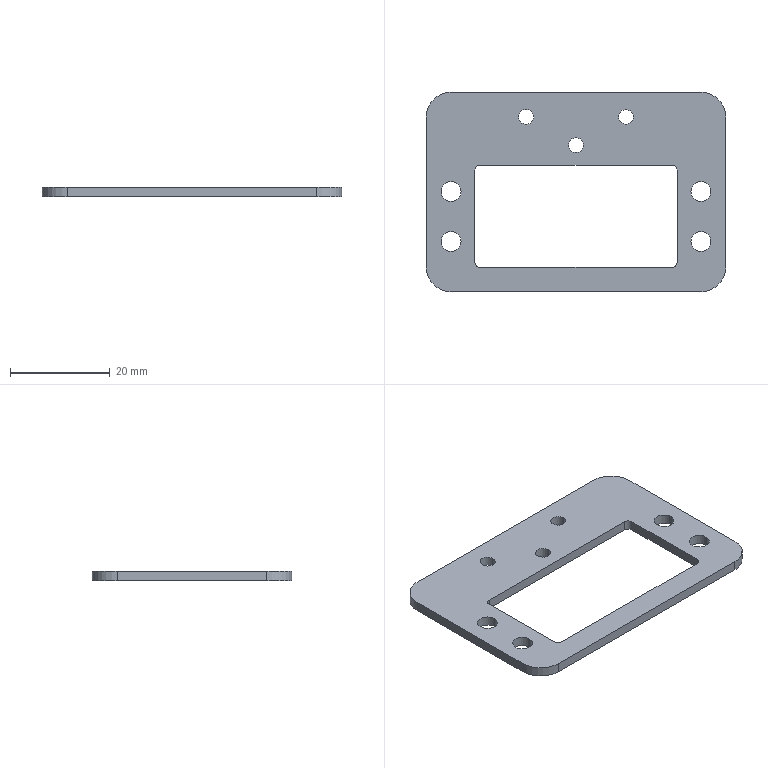Part | SolidWorks | features ICE 3, Extrusion 1 | 1 solid | 32 faces | box 60 x 40 x 2 mm | volume 2957 mm3 | cylinder 22 | plane 10 | commonest cylinder face diameters 4 x8 2 x4 10 x4 2.944 x2 3 x2 3.025 x2
STEP:
#1=CARTESIAN_POINT('',(25.172,6.576,0.));
#2=VERTEX_POINT('',#1);
#3=CARTESIAN_POINT('',(29.172,6.576,0.));
#4=VERTEX_POINT('',#3);
#5=CARTESIAN_POINT('',(27.172,6.576,0.));
#6=DIRECTION('',(0.,0.,1.));
#7=DIRECTION('',(1.,0.,0.));
#8=AXIS2_PLACEMENT_3D('',#5,#6,#7);
#9=CIRCLE('',#8,2.);
#10=EDGE_CURVE('',#2,#4,#9,.T.);
#11=ORIENTED_EDGE('',*,*,#10,.F.);
#12=CARTESIAN_POINT('',(25.172,6.576,2.));
#13=VERTEX_POINT('',#12);
#14=CARTESIAN_POINT('',(25.172,6.576,0.));
#15=DIRECTION('',(0.,0.,1.));
#16=VECTOR('',#15,1000.);
#17=LINE('',#14,#16);
#18=EDGE_CURVE('',#2,#13,#17,.T.);
#19=ORIENTED_EDGE('',*,*,#18,.T.);
#20=CARTESIAN_POINT('',(29.172,6.576,2.));
#21=VERTEX_POINT('',#20);
#22=CARTESIAN_POINT('',(27.172,6.576,2.));
#23=DIRECTION('',(0.,0.,1.));
#24=DIRECTION('',(1.,0.,0.));
#25=AXIS2_PLACEMENT_3D('',#22,#23,#24);
#26=CIRCLE('',#25,2.);
#27=EDGE_CURVE('',#13,#21,#26,.T.);
#28=ORIENTED_EDGE('',*,*,#27,.T.);
#29=CARTESIAN_POINT('',(29.172,6.576,0.));
#30=DIRECTION('',(0.,0.,1.));
#31=VECTOR('',#30,1000.);
#32=LINE('',#29,#31);
#33=EDGE_CURVE('',#4,#21,#32,.T.);
#34=ORIENTED_EDGE('',*,*,#33,.F.);
#35=EDGE_LOOP('',(#11,#19,#28,#34));
#36=FACE_OUTER_BOUND('',#35,.T.);
#37=CARTESIAN_POINT('',(27.172,6.576,0.));
#38=DIRECTION('',(0.,0.,1.));
#39=DIRECTION('',(1.,0.,0.));
#40=AXIS2_PLACEMENT_3D('',#37,#38,#39);
#41=CYLINDRICAL_SURFACE('',#40,2.);
#42=ADVANCED_FACE('',(#36),#41,.F.);
#43=CARTESIAN_POINT('',(-24.859,-3.424,0.));
#44=VERTEX_POINT('',#43);
#45=CARTESIAN_POINT('',(-20.859,-3.424,0.));
#46=VERTEX_POINT('',#45);
#47=CARTESIAN_POINT('',(-22.859,-3.424,0.));
#48=DIRECTION('',(0.,0.,1.));
#49=DIRECTION('',(-1.,0.,0.));
#50=AXIS2_PLACEMENT_3D('',#47,#48,#49);
#51=CIRCLE('',#50,2.);
#52=EDGE_CURVE('',#44,#46,#51,.T.);
#53=ORIENTED_EDGE('',*,*,#52,.F.);
#54=CARTESIAN_POINT('',(-24.859,-3.424,2.));
#55=VERTEX_POINT('',#54);
#56=CARTESIAN_POINT('',(-24.859,-3.424,0.));
#57=DIRECTION('',(0.,0.,1.));
#58=VECTOR('',#57,1000.);
#59=LINE('',#56,#58);
#60=EDGE_CURVE('',#44,#55,#59,.T.);
#61=ORIENTED_EDGE('',*,*,#60,.T.);
#62=CARTESIAN_POINT('',(-20.859,-3.424,2.));
#63=VERTEX_POINT('',#62);
#64=CARTESIAN_POINT('',(-22.859,-3.424,2.));
#65=DIRECTION('',(0.,0.,1.));
#66=DIRECTION('',(-1.,0.,0.));
#67=AXIS2_PLACEMENT_3D('',#64,#65,#66);
#68=CIRCLE('',#67,2.);
#69=EDGE_CURVE('',#55,#63,#68,.T.);
#70=ORIENTED_EDGE('',*,*,#69,.T.);
#71=CARTESIAN_POINT('',(-20.859,-3.424,0.));
#72=DIRECTION('',(0.,0.,1.));
#73=VECTOR('',#72,1000.);
#74=LINE('',#71,#73);
#75=EDGE_CURVE('',#46,#63,#74,.T.);
#76=ORIENTED_EDGE('',*,*,#75,.F.);
#77=EDGE_LOOP('',(#53,#61,#70,#76));
#78=FACE_OUTER_BOUND('',#77,.T.);
#79=CARTESIAN_POINT('',(-22.859,-3.424,0.));
#80=DIRECTION('',(0.,0.,1.));
#81=DIRECTION('',(1.,0.,0.));
#82=AXIS2_PLACEMENT_3D('',#79,#80,#81);
#83=CYLINDRICAL_SURFACE('',#82,2.);
#84=ADVANCED_FACE('',(#78),#83,.F.);
#85=CARTESIAN_POINT('',(-24.859,6.576,0.));
#86=VERTEX_POINT('',#85);
#87=CARTESIAN_POINT('',(-20.859,6.576,0.));
#88=VERTEX_POINT('',#87);
#89=CARTESIAN_POINT('',(-22.859,6.576,0.));
#90=DIRECTION('',(0.,0.,1.));
#91=DIRECTION('',(-1.,0.,0.));
#92=AXIS2_PLACEMENT_3D('',#89,#90,#91);
#93=CIRCLE('',#92,2.);
#94=EDGE_CURVE('',#86,#88,#93,.T.);
#95=ORIENTED_EDGE('',*,*,#94,.F.);
#96=CARTESIAN_POINT('',(-24.859,6.576,2.));
#97=VERTEX_POINT('',#96);
#98=CARTESIAN_POINT('',(-24.859,6.576,0.));
#99=DIRECTION('',(0.,0.,1.));
#100=VECTOR('',#99,1000.);
#101=LINE('',#98,#100);
#102=EDGE_CURVE('',#86,#97,#101,.T.);
#103=ORIENTED_EDGE('',*,*,#102,.T.);
#104=CARTESIAN_POINT('',(-20.859,6.576,2.));
#105=VERTEX_POINT('',#104);
#106=CARTESIAN_POINT('',(-22.859,6.576,2.));
#107=DIRECTION('',(0.,0.,1.));
#108=DIRECTION('',(-1.,0.,0.));
#109=AXIS2_PLACEMENT_3D('',#106,#107,#108);
#110=CIRCLE('',#109,2.);
#111=EDGE_CURVE('',#97,#105,#110,.T.);
#112=ORIENTED_EDGE('',*,*,#111,.T.);
#113=CARTESIAN_POINT('',(-20.859,6.576,0.));
#114=DIRECTION('',(0.,0.,1.));
#115=VECTOR('',#114,1000.);
#116=LINE('',#113,#115);
#117=EDGE_CURVE('',#88,#105,#116,.T.);
#118=ORIENTED_EDGE('',*,*,#117,.F.);
#119=EDGE_LOOP('',(#95,#103,#112,#118));
#120=FACE_OUTER_BOUND('',#119,.T.);
#121=CARTESIAN_POINT('',(-22.859,6.576,0.));
#122=DIRECTION('',(0.,0.,1.));
#123=DIRECTION('',(1.,0.,0.));
#124=AXIS2_PLACEMENT_3D('',#121,#122,#123);
#125=CYLINDRICAL_SURFACE('',#124,2.);
#126=ADVANCED_FACE('',(#120),#125,.F.);
#127=CARTESIAN_POINT('',(25.172,-3.424,0.));
#128=VERTEX_POINT('',#127);
#129=CARTESIAN_POINT('',(29.172,-3.424,0.));
#130=VERTEX_POINT('',#129);
#131=CARTESIAN_POINT('',(27.172,-3.424,0.));
#132=DIRECTION('',(0.,0.,1.));
#133=DIRECTION('',(1.,0.,0.));
#134=AXIS2_PLACEMENT_3D('',#131,#132,#133);
#135=CIRCLE('',#134,2.);
#136=EDGE_CURVE('',#128,#130,#135,.T.);
#137=ORIENTED_EDGE('',*,*,#136,.F.);
#138=CARTESIAN_POINT('',(25.172,-3.424,2.));
#139=VERTEX_POINT('',#138);
#140=CARTESIAN_POINT('',(25.172,-3.424,0.));
#141=DIRECTION('',(0.,0.,1.));
#142=VECTOR('',#141,1000.);
#143=LINE('',#140,#142);
#144=EDGE_CURVE('',#128,#139,#143,.T.);
#145=ORIENTED_EDGE('',*,*,#144,.T.);
#146=CARTESIAN_POINT('',(29.172,-3.424,2.));
#147=VERTEX_POINT('',#146);
#148=CARTESIAN_POINT('',(27.172,-3.424,2.));
#149=DIRECTION('',(0.,0.,1.));
#150=DIRECTION('',(1.,0.,0.));
#151=AXIS2_PLACEMENT_3D('',#148,#149,#150);
#152=CIRCLE('',#151,2.);
#153=EDGE_CURVE('',#139,#147,#152,.T.);
#154=ORIENTED_EDGE('',*,*,#153,.T.);
#155=CARTESIAN_POINT('',(29.172,-3.424,0.));
#156=DIRECTION('',(0.,0.,1.));
#157=VECTOR('',#156,1000.);
#158=LINE('',#155,#157);
#159=EDGE_CURVE('',#130,#147,#158,.T.);
#160=ORIENTED_EDGE('',*,*,#159,.F.);
#161=EDGE_LOOP('',(#137,#145,#154,#160));
#162=FACE_OUTER_BOUND('',#161,.T.);
#163=CARTESIAN_POINT('',(27.172,-3.424,0.));
#164=DIRECTION('',(0.,0.,1.));
#165=DIRECTION('',(1.,0.,0.));
#166=AXIS2_PLACEMENT_3D('',#163,#164,#165);
#167=CYLINDRICAL_SURFACE('',#166,2.);
#168=ADVANCED_FACE('',(#162),#167,.F.);
#169=CARTESIAN_POINT('',(0.6565,15.876,0.));
#170=VERTEX_POINT('',#169);
#171=CARTESIAN_POINT('',(3.657,15.876,0.));
#172=VERTEX_POINT('',#171);
#173=CARTESIAN_POINT('',(2.157,15.876,0.));
#174=DIRECTION('',(0.,0.,1.));
#175=DIRECTION('',(1.,0.,0.));
#176=AXIS2_PLACEMENT_3D('',#173,#174,#175);
#177=CIRCLE('',#176,1.5);
#178=EDGE_CURVE('',#170,#172,#177,.T.);
#179=ORIENTED_EDGE('',*,*,#178,.F.);
#180=CARTESIAN_POINT('',(0.6565,15.876,2.));
#181=VERTEX_POINT('',#180);
#182=CARTESIAN_POINT('',(0.6565,15.876,0.));
#183=DIRECTION('',(0.,0.,1.));
#184=VECTOR('',#183,1000.);
#185=LINE('',#182,#184);
#186=EDGE_CURVE('',#170,#181,#185,.T.);
#187=ORIENTED_EDGE('',*,*,#186,.T.);
#188=CARTESIAN_POINT('',(3.657,15.876,2.));
#189=VERTEX_POINT('',#188);
#190=CARTESIAN_POINT('',(2.157,15.876,2.));
#191=DIRECTION('',(0.,0.,1.));
#192=DIRECTION('',(1.,0.,0.));
#193=AXIS2_PLACEMENT_3D('',#190,#191,#192);
#194=CIRCLE('',#193,1.5);
#195=EDGE_CURVE('',#181,#189,#194,.T.);
#196=ORIENTED_EDGE('',*,*,#195,.T.);
#197=CARTESIAN_POINT('',(3.657,15.876,0.));
#198=DIRECTION('',(0.,0.,1.));
#199=VECTOR('',#198,1000.);
#200=LINE('',#197,#199);
#201=EDGE_CURVE('',#172,#189,#200,.T.);
#202=ORIENTED_EDGE('',*,*,#201,.F.);
#203=EDGE_LOOP('',(#179,#187,#196,#202));
#204=FACE_OUTER_BOUND('',#203,.T.);
#205=CARTESIAN_POINT('',(2.157,15.876,0.));
#206=DIRECTION('',(0.,0.,1.));
#207=DIRECTION('',(1.,0.,0.));
#208=AXIS2_PLACEMENT_3D('',#205,#206,#207);
#209=CYLINDRICAL_SURFACE('',#208,1.5);
#210=ADVANCED_FACE('',(#204),#209,.F.);
#211=CARTESIAN_POINT('',(10.684,21.526,0.));
#212=VERTEX_POINT('',#211);
#213=CARTESIAN_POINT('',(13.629,21.526,0.));
#214=VERTEX_POINT('',#213);
#215=CARTESIAN_POINT('',(12.157,21.526,0.));
#216=DIRECTION('',(0.,0.,1.));
#217=DIRECTION('',(1.,0.,0.));
#218=AXIS2_PLACEMENT_3D('',#215,#216,#217);
#219=CIRCLE('',#218,1.472);
#220=EDGE_CURVE('',#212,#214,#219,.T.);
#221=ORIENTED_EDGE('',*,*,#220,.F.);
#222=CARTESIAN_POINT('',(10.684,21.526,2.));
#223=VERTEX_POINT('',#222);
#224=CARTESIAN_POINT('',(10.684,21.526,0.));
#225=DIRECTION('',(0.,0.,1.));
#226=VECTOR('',#225,1000.);
#227=LINE('',#224,#226);
#228=EDGE_CURVE('',#212,#223,#227,.T.);
#229=ORIENTED_EDGE('',*,*,#228,.T.);
#230=CARTESIAN_POINT('',(13.629,21.526,2.));
#231=VERTEX_POINT('',#230);
#232=CARTESIAN_POINT('',(12.157,21.526,2.));
#233=DIRECTION('',(0.,0.,1.));
#234=DIRECTION('',(1.,0.,0.));
#235=AXIS2_PLACEMENT_3D('',#232,#233,#234);
#236=CIRCLE('',#235,1.472);
#237=EDGE_CURVE('',#223,#231,#236,.T.);
#238=ORIENTED_EDGE('',*,*,#237,.T.);
#239=CARTESIAN_POINT('',(13.629,21.526,0.));
#240=DIRECTION('',(0.,0.,1.));
#241=VECTOR('',#240,1000.);
#242=LINE('',#239,#241);
#243=EDGE_CURVE('',#214,#231,#242,.T.);
#244=ORIENTED_EDGE('',*,*,#243,.F.);
#245=EDGE_LOOP('',(#221,#229,#238,#244));
#246=FACE_OUTER_BOUND('',#245,.T.);
#247=CARTESIAN_POINT('',(12.157,21.526,0.));
#248=DIRECTION('',(0.,0.,1.));
#249=DIRECTION('',(1.,0.,0.));
#250=AXIS2_PLACEMENT_3D('',#247,#248,#249);
#251=CYLINDRICAL_SURFACE('',#250,1.472);
#252=ADVANCED_FACE('',(#246),#251,.F.);
#253=CARTESIAN_POINT('',(-9.356,21.526,0.));
#254=VERTEX_POINT('',#253);
#255=CARTESIAN_POINT('',(-6.331,21.526,0.));
#256=VERTEX_POINT('',#255);
#257=CARTESIAN_POINT('',(-7.843,21.526,0.));
#258=DIRECTION('',(0.,0.,1.));
#259=DIRECTION('',(1.,0.,0.));
#260=AXIS2_PLACEMENT_3D('',#257,#258,#259);
#261=CIRCLE('',#260,1.512);
#262=EDGE_CURVE('',#254,#256,#261,.T.);
#263=ORIENTED_EDGE('',*,*,#262,.F.);
#264=CARTESIAN_POINT('',(-9.356,21.526,2.));
#265=VERTEX_POINT('',#264);
#266=CARTESIAN_POINT('',(-9.356,21.526,0.));
#267=DIRECTION('',(0.,0.,1.));
#268=VECTOR('',#267,1000.);
#269=LINE('',#266,#268);
#270=EDGE_CURVE('',#254,#265,#269,.T.);
#271=ORIENTED_EDGE('',*,*,#270,.T.);
#272=CARTESIAN_POINT('',(-6.331,21.526,2.));
#273=VERTEX_POINT('',#272);
#274=CARTESIAN_POINT('',(-7.843,21.526,2.));
#275=DIRECTION('',(0.,0.,1.));
#276=DIRECTION('',(1.,0.,0.));
#277=AXIS2_PLACEMENT_3D('',#274,#275,#276);
#278=CIRCLE('',#277,1.512);
#279=EDGE_CURVE('',#265,#273,#278,.T.);
#280=ORIENTED_EDGE('',*,*,#279,.T.);
#281=CARTESIAN_POINT('',(-6.331,21.526,0.));
#282=DIRECTION('',(0.,0.,1.));
#283=VECTOR('',#282,1000.);
#284=LINE('',#281,#283);
#285=EDGE_CURVE('',#256,#273,#284,.T.);
#286=ORIENTED_EDGE('',*,*,#285,.F.);
#287=EDGE_LOOP('',(#263,#271,#280,#286));
#288=FACE_OUTER_BOUND('',#287,.T.);
#289=CARTESIAN_POINT('',(-7.843,21.526,0.));
#290=DIRECTION('',(0.,0.,1.));
#291=DIRECTION('',(1.,0.,0.));
#292=AXIS2_PLACEMENT_3D('',#289,#290,#291);
#293=CYLINDRICAL_SURFACE('',#292,1.512);
#294=ADVANCED_FACE('',(#288),#293,.F.);
#295=CARTESIAN_POINT('',(27.157,-13.514,0.));
#296=VERTEX_POINT('',#295);
#297=CARTESIAN_POINT('',(32.157,-8.514,0.));
#298=VERTEX_POINT('',#297);
#299=CARTESIAN_POINT('',(27.157,-8.514,0.));
#300=DIRECTION('',(0.,0.,1.));
#301=DIRECTION('',(1.,0.,0.));
#302=AXIS2_PLACEMENT_3D('',#299,#300,#301);
#303=CIRCLE('',#302,5.);
#304=EDGE_CURVE('',#296,#298,#303,.T.);
#305=ORIENTED_EDGE('',*,*,#304,.T.);
#306=CARTESIAN_POINT('',(32.157,-8.514,2.));
#307=VERTEX_POINT('',#306);
#308=CARTESIAN_POINT('',(32.157,-8.514,2.));
#309=DIRECTION('',(0.,0.,-1.));
#310=VECTOR('',#309,1000.);
#311=LINE('',#308,#310);
#312=EDGE_CURVE('',#307,#298,#311,.T.);
#313=ORIENTED_EDGE('',*,*,#312,.F.);
#314=CARTESIAN_POINT('',(27.157,-13.514,2.));
#315=VERTEX_POINT('',#314);
#316=CARTESIAN_POINT('',(27.157,-8.514,2.));
#317=DIRECTION('',(0.,0.,1.));
#318=DIRECTION('',(1.,0.,0.));
#319=AXIS2_PLACEMENT_3D('',#316,#317,#318);
#320=CIRCLE('',#319,5.);
#321=EDGE_CURVE('',#315,#307,#320,.T.);
#322=ORIENTED_EDGE('',*,*,#321,.F.);
#323=CARTESIAN_POINT('',(27.157,-13.514,2.));
#324=DIRECTION('',(0.,0.,-1.));
#325=VECTOR('',#324,1000.);
#326=LINE('',#323,#325);
#327=EDGE_CURVE('',#315,#296,#326,.T.);
#328=ORIENTED_EDGE('',*,*,#327,.T.);
#329=EDGE_LOOP('',(#305,#313,#322,#328));
#330=FACE_OUTER_BOUND('',#329,.T.);
#331=CARTESIAN_POINT('',(27.157,-8.514,2.));
#332=DIRECTION('',(0.,0.,-1.));
#333=DIRECTION('',(-1.,0.,0.));
#334=AXIS2_PLACEMENT_3D('',#331,#332,#333);
#335=CYLINDRICAL_SURFACE('',#334,5.);
#336=ADVANCED_FACE('',(#330),#335,.T.);
#337=CARTESIAN_POINT('',(32.157,21.486,0.));
#338=VERTEX_POINT('',#337);
#339=CARTESIAN_POINT('',(32.157,21.486,0.));
#340=DIRECTION('',(0.,1.,0.));
#341=VECTOR('',#340,1000.);
#342=LINE('',#339,#341);
#343=EDGE_CURVE('',#298,#338,#342,.T.);
#344=ORIENTED_EDGE('',*,*,#343,.T.);
#345=CARTESIAN_POINT('',(32.157,21.486,2.));
#346=VERTEX_POINT('',#345);
#347=CARTESIAN_POINT('',(32.157,21.486,2.));
#348=DIRECTION('',(0.,0.,-1.));
#349=VECTOR('',#348,1000.);
#350=LINE('',#347,#349);
#351=EDGE_CURVE('',#346,#338,#350,.T.);
#352=ORIENTED_EDGE('',*,*,#351,.F.);
#353=CARTESIAN_POINT('',(32.157,21.486,2.));
#354=DIRECTION('',(0.,1.,0.));
#355=VECTOR('',#354,1000.);
#356=LINE('',#353,#355);
#357=EDGE_CURVE('',#307,#346,#356,.T.);
#358=ORIENTED_EDGE('',*,*,#357,.F.);
#359=ORIENTED_EDGE('',*,*,#312,.T.);
#360=EDGE_LOOP('',(#344,#352,#358,#359));
#361=FACE_OUTER_BOUND('',#360,.T.);
#362=CARTESIAN_POINT('',(32.157,21.486,2.));
#363=DIRECTION('',(-1.,0.,0.));
#364=DIRECTION('',(0.,0.,1.));
#365=AXIS2_PLACEMENT_3D('',#362,#363,#364);
#366=PLANE('',#365);
#367=ADVANCED_FACE('',(#361),#366,.F.);
#368=CARTESIAN_POINT('',(27.157,26.486,0.));
#369=VERTEX_POINT('',#368);
#370=CARTESIAN_POINT('',(27.157,21.486,0.));
#371=DIRECTION('',(0.,0.,1.));
#372=DIRECTION('',(-1.,0.,0.));
#373=AXIS2_PLACEMENT_3D('',#370,#371,#372);
#374=CIRCLE('',#373,5.);
#375=EDGE_CURVE('',#338,#369,#374,.T.);
#376=ORIENTED_EDGE('',*,*,#375,.T.);
#377=CARTESIAN_POINT('',(27.157,26.486,2.));
#378=VERTEX_POINT('',#377);
#379=CARTESIAN_POINT('',(27.157,26.486,2.));
#380=DIRECTION('',(0.,0.,-1.));
#381=VECTOR('',#380,1000.);
#382=LINE('',#379,#381);
#383=EDGE_CURVE('',#378,#369,#382,.T.);
#384=ORIENTED_EDGE('',*,*,#383,.F.);
#385=CARTESIAN_POINT('',(27.157,21.486,2.));
#386=DIRECTION('',(0.,0.,1.));
#387=DIRECTION('',(-1.,0.,0.));
#388=AXIS2_PLACEMENT_3D('',#385,#386,#387);
#389=CIRCLE('',#388,5.);
#390=EDGE_CURVE('',#346,#378,#389,.T.);
#391=ORIENTED_EDGE('',*,*,#390,.F.);
#392=ORIENTED_EDGE('',*,*,#351,.T.);
#393=EDGE_LOOP('',(#376,#384,#391,#392));
#394=FACE_OUTER_BOUND('',#393,.T.);
#395=CARTESIAN_POINT('',(27.157,21.486,2.));
#396=DIRECTION('',(0.,0.,-1.));
#397=DIRECTION('',(-1.,0.,0.));
#398=AXIS2_PLACEMENT_3D('',#395,#396,#397);
#399=CYLINDRICAL_SURFACE('',#398,5.);
#400=ADVANCED_FACE('',(#394),#399,.T.);
#401=CARTESIAN_POINT('',(-22.843,26.486,0.));
#402=VERTEX_POINT('',#401);
#403=CARTESIAN_POINT('',(-22.843,26.486,0.));
#404=DIRECTION('',(-1.,0.,0.));
#405=VECTOR('',#404,1000.);
#406=LINE('',#403,#405);
#407=EDGE_CURVE('',#369,#402,#406,.T.);
#408=ORIENTED_EDGE('',*,*,#407,.T.);
#409=CARTESIAN_POINT('',(-22.843,26.486,2.));
#410=VERTEX_POINT('',#409);
#411=CARTESIAN_POINT('',(-22.843,26.486,2.));
#412=DIRECTION('',(0.,0.,-1.));
#413=VECTOR('',#412,1000.);
#414=LINE('',#411,#413);
#415=EDGE_CURVE('',#410,#402,#414,.T.);
#416=ORIENTED_EDGE('',*,*,#415,.F.);
#417=CARTESIAN_POINT('',(-22.843,26.486,2.));
#418=DIRECTION('',(-1.,0.,0.));
#419=VECTOR('',#418,1000.);
#420=LINE('',#417,#419);
#421=EDGE_CURVE('',#378,#410,#420,.T.);
#422=ORIENTED_EDGE('',*,*,#421,.F.);
#423=ORIENTED_EDGE('',*,*,#383,.T.);
#424=EDGE_LOOP('',(#408,#416,#422,#423));
#425=FACE_OUTER_BOUND('',#424,.T.);
#426=CARTESIAN_POINT('',(-22.843,26.486,2.));
#427=DIRECTION('',(0.,-1.,0.));
#428=DIRECTION('',(0.,0.,-1.));
#429=AXIS2_PLACEMENT_3D('',#426,#427,#428);
#430=PLANE('',#429);
#431=ADVANCED_FACE('',(#425),#430,.F.);
#432=CARTESIAN_POINT('',(-27.843,21.486,0.));
#433=VERTEX_POINT('',#432);
#434=CARTESIAN_POINT('',(-22.843,21.486,0.));
#435=DIRECTION('',(0.,0.,1.));
#436=DIRECTION('',(1.,0.,0.));
#437=AXIS2_PLACEMENT_3D('',#434,#435,#436);
#438=CIRCLE('',#437,5.);
#439=EDGE_CURVE('',#402,#433,#438,.T.);
#440=ORIENTED_EDGE('',*,*,#439,.T.);
#441=CARTESIAN_POINT('',(-27.843,21.486,2.));
#442=VERTEX_POINT('',#441);
#443=CARTESIAN_POINT('',(-27.843,21.486,2.));
#444=DIRECTION('',(0.,0.,-1.));
#445=VECTOR('',#444,1000.);
#446=LINE('',#443,#445);
#447=EDGE_CURVE('',#442,#433,#446,.T.);
#448=ORIENTED_EDGE('',*,*,#447,.F.);
#449=CARTESIAN_POINT('',(-22.843,21.486,2.));
#450=DIRECTION('',(0.,0.,1.));
#451=DIRECTION('',(1.,0.,0.));
#452=AXIS2_PLACEMENT_3D('',#449,#450,#451);
#453=CIRCLE('',#452,5.);
#454=EDGE_CURVE('',#410,#442,#453,.T.);
#455=ORIENTED_EDGE('',*,*,#454,.F.);
#456=ORIENTED_EDGE('',*,*,#415,.T.);
#457=EDGE_LOOP('',(#440,#448,#455,#456));
#458=FACE_OUTER_BOUND('',#457,.T.);
#459=CARTESIAN_POINT('',(-22.843,21.486,2.));
#460=DIRECTION('',(0.,0.,-1.));
#461=DIRECTION('',(-1.,0.,0.));
#462=AXIS2_PLACEMENT_3D('',#459,#460,#461);
#463=CYLINDRICAL_SURFACE('',#462,5.);
#464=ADVANCED_FACE('',(#458),#463,.T.);
#465=CARTESIAN_POINT('',(-27.843,-8.514,0.));
#466=VERTEX_POINT('',#465);
#467=CARTESIAN_POINT('',(-27.843,21.486,0.));
#468=DIRECTION('',(0.,-1.,0.));
#469=VECTOR('',#468,1000.);
#470=LINE('',#467,#469);
#471=EDGE_CURVE('',#433,#466,#470,.T.);
#472=ORIENTED_EDGE('',*,*,#471,.T.);
#473=CARTESIAN_POINT('',(-27.843,-8.514,2.));
#474=VERTEX_POINT('',#473);
#475=CARTESIAN_POINT('',(-27.843,-8.514,2.));
#476=DIRECTION('',(0.,0.,-1.));
#477=VECTOR('',#476,1000.);
#478=LINE('',#475,#477);
#479=EDGE_CURVE('',#474,#466,#478,.T.);
#480=ORIENTED_EDGE('',*,*,#479,.F.);
#481=CARTESIAN_POINT('',(-27.843,21.486,2.));
#482=DIRECTION('',(0.,-1.,0.));
#483=VECTOR('',#482,1000.);
#484=LINE('',#481,#483);
#485=EDGE_CURVE('',#442,#474,#484,.T.);
#486=ORIENTED_EDGE('',*,*,#485,.F.);
#487=ORIENTED_EDGE('',*,*,#447,.T.);
#488=EDGE_LOOP('',(#472,#480,#486,#487));
#489=FACE_OUTER_BOUND('',#488,.T.);
#490=CARTESIAN_POINT('',(-27.843,21.486,2.));
#491=DIRECTION('',(1.,0.,0.));
#492=DIRECTION('',(0.,0.,-1.));
#493=AXIS2_PLACEMENT_3D('',#490,#491,#492);
#494=PLANE('',#493);
#495=ADVANCED_FACE('',(#489),#494,.F.);
#496=CARTESIAN_POINT('',(-22.843,-13.514,0.));
#497=VERTEX_POINT('',#496);
#498=CARTESIAN_POINT('',(-22.843,-8.514,0.));
#499=DIRECTION('',(0.,0.,1.));
#500=DIRECTION('',(1.,0.,0.));
#501=AXIS2_PLACEMENT_3D('',#498,#499,#500);
#502=CIRCLE('',#501,5.);
#503=EDGE_CURVE('',#466,#497,#502,.T.);
#504=ORIENTED_EDGE('',*,*,#503,.T.);
#505=CARTESIAN_POINT('',(-22.843,-13.514,2.));
#506=VERTEX_POINT('',#505);
#507=CARTESIAN_POINT('',(-22.843,-13.514,2.));
#508=DIRECTION('',(0.,0.,-1.));
#509=VECTOR('',#508,1000.);
#510=LINE('',#507,#509);
#511=EDGE_CURVE('',#506,#497,#510,.T.);
#512=ORIENTED_EDGE('',*,*,#511,.F.);
#513=CARTESIAN_POINT('',(-22.843,-8.514,2.));
#514=DIRECTION('',(0.,0.,1.));
#515=DIRECTION('',(1.,0.,0.));
#516=AXIS2_PLACEMENT_3D('',#513,#514,#515);
#517=CIRCLE('',#516,5.);
#518=EDGE_CURVE('',#474,#506,#517,.T.);
#519=ORIENTED_EDGE('',*,*,#518,.F.);
#520=ORIENTED_EDGE('',*,*,#479,.T.);
#521=EDGE_LOOP('',(#504,#512,#519,#520));
#522=FACE_OUTER_BOUND('',#521,.T.);
#523=CARTESIAN_POINT('',(-22.843,-8.514,2.));
#524=DIRECTION('',(0.,0.,-1.));
#525=DIRECTION('',(-1.,0.,0.));
#526=AXIS2_PLACEMENT_3D('',#523,#524,#525);
#527=CYLINDRICAL_SURFACE('',#526,5.);
#528=ADVANCED_FACE('',(#522),#527,.T.);
#529=CARTESIAN_POINT('',(-22.843,-13.514,0.));
#530=DIRECTION('',(1.,0.,0.));
#531=VECTOR('',#530,1000.);
#532=LINE('',#529,#531);
#533=EDGE_CURVE('',#497,#296,#532,.T.);
#534=ORIENTED_EDGE('',*,*,#533,.T.);
#535=ORIENTED_EDGE('',*,*,#327,.F.);
#536=CARTESIAN_POINT('',(-22.843,-13.514,2.));
#537=DIRECTION('',(1.,0.,0.));
#538=VECTOR('',#537,1000.);
#539=LINE('',#536,#538);
#540=EDGE_CURVE('',#506,#315,#539,.T.);
#541=ORIENTED_EDGE('',*,*,#540,.F.);
#542=ORIENTED_EDGE('',*,*,#511,.T.);
#543=EDGE_LOOP('',(#534,#535,#541,#542));
#544=FACE_OUTER_BOUND('',#543,.T.);
#545=CARTESIAN_POINT('',(-22.843,-13.514,2.));
#546=DIRECTION('',(0.,1.,0.));
#547=DIRECTION('',(0.,0.,1.));
#548=AXIS2_PLACEMENT_3D('',#545,#546,#547);
#549=PLANE('',#548);
#550=ADVANCED_FACE('',(#544),#549,.F.);
#551=CARTESIAN_POINT('',(27.172,6.576,2.));
#552=DIRECTION('',(0.,0.,1.));
#553=DIRECTION('',(1.,0.,0.));
#554=AXIS2_PLACEMENT_3D('',#551,#552,#553);
#555=CIRCLE('',#554,2.);
#556=EDGE_CURVE('',#21,#13,#555,.T.);
#557=ORIENTED_EDGE('',*,*,#556,.F.);
#558=ORIENTED_EDGE('',*,*,#27,.F.);
#559=EDGE_LOOP('',(#557,#558));
#560=FACE_BOUND('',#559,.T.);
#561=CARTESIAN_POINT('',(-22.859,-3.424,2.));
#562=DIRECTION('',(0.,0.,1.));
#563=DIRECTION('',(-1.,0.,0.));
#564=AXIS2_PLACEMENT_3D('',#561,#562,#563);
#565=CIRCLE('',#564,2.);
#566=EDGE_CURVE('',#63,#55,#565,.T.);
#567=ORIENTED_EDGE('',*,*,#566,.F.);
#568=ORIENTED_EDGE('',*,*,#69,.F.);
#569=EDGE_LOOP('',(#567,#568));
#570=FACE_BOUND('',#569,.T.);
#571=CARTESIAN_POINT('',(-22.859,6.576,2.));
#572=DIRECTION('',(0.,0.,1.));
#573=DIRECTION('',(-1.,0.,0.));
#574=AXIS2_PLACEMENT_3D('',#571,#572,#573);
#575=CIRCLE('',#574,2.);
#576=EDGE_CURVE('',#105,#97,#575,.T.);
#577=ORIENTED_EDGE('',*,*,#576,.F.);
#578=ORIENTED_EDGE('',*,*,#111,.F.);
#579=EDGE_LOOP('',(#577,#578));
#580=FACE_BOUND('',#579,.T.);
#581=CARTESIAN_POINT('',(27.172,-3.424,2.));
#582=DIRECTION('',(0.,0.,1.));
#583=DIRECTION('',(1.,0.,0.));
#584=AXIS2_PLACEMENT_3D('',#581,#582,#583);
#585=CIRCLE('',#584,2.);
#586=EDGE_CURVE('',#147,#139,#585,.T.);
#587=ORIENTED_EDGE('',*,*,#586,.F.);
#588=ORIENTED_EDGE('',*,*,#153,.F.);
#589=EDGE_LOOP('',(#587,#588));
#590=FACE_BOUND('',#589,.T.);
#591=CARTESIAN_POINT('',(2.157,15.876,2.));
#592=DIRECTION('',(0.,0.,1.));
#593=DIRECTION('',(1.,0.,0.));
#594=AXIS2_PLACEMENT_3D('',#591,#592,#593);
#595=CIRCLE('',#594,1.5);
#596=EDGE_CURVE('',#189,#181,#595,.T.);
#597=ORIENTED_EDGE('',*,*,#596,.F.);
#598=ORIENTED_EDGE('',*,*,#195,.F.);
#599=EDGE_LOOP('',(#597,#598));
#600=FACE_BOUND('',#599,.T.);
#601=CARTESIAN_POINT('',(12.157,21.526,2.));
#602=DIRECTION('',(0.,0.,1.));
#603=DIRECTION('',(1.,0.,0.));
#604=AXIS2_PLACEMENT_3D('',#601,#602,#603);
#605=CIRCLE('',#604,1.472);
#606=EDGE_CURVE('',#231,#223,#605,.T.);
#607=ORIENTED_EDGE('',*,*,#606,.F.);
#608=ORIENTED_EDGE('',*,*,#237,.F.);
#609=EDGE_LOOP('',(#607,#608));
#610=FACE_BOUND('',#609,.T.);
#611=CARTESIAN_POINT('',(-7.843,21.526,2.));
#612=DIRECTION('',(0.,0.,1.));
#613=DIRECTION('',(1.,0.,0.));
#614=AXIS2_PLACEMENT_3D('',#611,#612,#613);
#615=CIRCLE('',#614,1.512);
#616=EDGE_CURVE('',#273,#265,#615,.T.);
#617=ORIENTED_EDGE('',*,*,#616,.F.);
#618=ORIENTED_EDGE('',*,*,#279,.F.);
#619=EDGE_LOOP('',(#617,#618));
#620=FACE_BOUND('',#619,.T.);
#621=CARTESIAN_POINT('',(-18.076,-7.624,2.));
#622=VERTEX_POINT('',#621);
#623=CARTESIAN_POINT('',(-17.076,-8.624,2.));
#624=VERTEX_POINT('',#623);
#625=CARTESIAN_POINT('',(-17.076,-7.624,2.));
#626=DIRECTION('',(0.,0.,1.));
#627=DIRECTION('',(1.,0.,0.));
#628=AXIS2_PLACEMENT_3D('',#625,#626,#627);
#629=CIRCLE('',#628,1.);
#630=EDGE_CURVE('',#622,#624,#629,.T.);
#631=ORIENTED_EDGE('',*,*,#630,.F.);
#632=CARTESIAN_POINT('',(-18.076,10.876,2.));
#633=VERTEX_POINT('',#632);
#634=CARTESIAN_POINT('',(-18.076,10.876,2.));
#635=DIRECTION('',(0.,-1.,0.));
#636=VECTOR('',#635,1000.);
#637=LINE('',#634,#636);
#638=EDGE_CURVE('',#633,#622,#637,.T.);
#639=ORIENTED_EDGE('',*,*,#638,.F.);
#640=CARTESIAN_POINT('',(-17.076,11.876,2.));
#641=VERTEX_POINT('',#640);
#642=CARTESIAN_POINT('',(-17.076,10.876,2.));
#643=DIRECTION('',(0.,0.,1.));
#644=DIRECTION('',(1.,0.,0.));
#645=AXIS2_PLACEMENT_3D('',#642,#643,#644);
#646=CIRCLE('',#645,1.);
#647=EDGE_CURVE('',#641,#633,#646,.T.);
#648=ORIENTED_EDGE('',*,*,#647,.F.);
#649=CARTESIAN_POINT('',(21.389,11.876,2.));
#650=VERTEX_POINT('',#649);
#651=CARTESIAN_POINT('',(-17.076,11.876,2.));
#652=DIRECTION('',(-1.,0.,0.));
#653=VECTOR('',#652,1000.);
#654=LINE('',#651,#653);
#655=EDGE_CURVE('',#650,#641,#654,.T.);
#656=ORIENTED_EDGE('',*,*,#655,.F.);
#657=CARTESIAN_POINT('',(22.389,10.876,2.));
#658=VERTEX_POINT('',#657);
#659=CARTESIAN_POINT('',(21.389,10.876,2.));
#660=DIRECTION('',(0.,0.,1.));
#661=DIRECTION('',(1.,0.,0.));
#662=AXIS2_PLACEMENT_3D('',#659,#660,#661);
#663=CIRCLE('',#662,1.);
#664=EDGE_CURVE('',#658,#650,#663,.T.);
#665=ORIENTED_EDGE('',*,*,#664,.F.);
#666=CARTESIAN_POINT('',(22.389,-7.624,2.));
#667=VERTEX_POINT('',#666);
#668=CARTESIAN_POINT('',(22.389,10.876,2.));
#669=DIRECTION('',(0.,1.,0.));
#670=VECTOR('',#669,1000.);
#671=LINE('',#668,#670);
#672=EDGE_CURVE('',#667,#658,#671,.T.);
#673=ORIENTED_EDGE('',*,*,#672,.F.);
#674=CARTESIAN_POINT('',(21.389,-8.624,2.));
#675=VERTEX_POINT('',#674);
#676=CARTESIAN_POINT('',(21.389,-7.624,2.));
#677=DIRECTION('',(0.,0.,1.));
#678=DIRECTION('',(1.,0.,0.));
#679=AXIS2_PLACEMENT_3D('',#676,#677,#678);
#680=CIRCLE('',#679,1.);
#681=EDGE_CURVE('',#675,#667,#680,.T.);
#682=ORIENTED_EDGE('',*,*,#681,.F.);
#683=CARTESIAN_POINT('',(-17.076,-8.624,2.));
#684=DIRECTION('',(1.,0.,0.));
#685=VECTOR('',#684,1000.);
#686=LINE('',#683,#685);
#687=EDGE_CURVE('',#624,#675,#686,.T.);
#688=ORIENTED_EDGE('',*,*,#687,.F.);
#689=EDGE_LOOP('',(#631,#639,#648,#656,#665,#673,#682,#688));
#690=FACE_BOUND('',#689,.T.);
#691=ORIENTED_EDGE('',*,*,#321,.T.);
#692=ORIENTED_EDGE('',*,*,#357,.T.);
#693=ORIENTED_EDGE('',*,*,#390,.T.);
#694=ORIENTED_EDGE('',*,*,#421,.T.);
#695=ORIENTED_EDGE('',*,*,#454,.T.);
#696=ORIENTED_EDGE('',*,*,#485,.T.);
#697=ORIENTED_EDGE('',*,*,#518,.T.);
#698=ORIENTED_EDGE('',*,*,#540,.T.);
#699=EDGE_LOOP('',(#691,#692,#693,#694,#695,#696,#697,#698));
#700=FACE_OUTER_BOUND('',#699,.T.);
#701=CARTESIAN_POINT('',(27.157,-8.514,2.));
#702=DIRECTION('',(0.,0.,1.));
#703=DIRECTION('',(1.,0.,0.));
#704=AXIS2_PLACEMENT_3D('',#701,#702,#703);
#705=PLANE('',#704);
#706=ADVANCED_FACE('',(#560,#570,#580,#590,#600,#610,#620,#690,#700),#705,.T.);
#707=CARTESIAN_POINT('',(27.172,6.576,0.));
#708=DIRECTION('',(0.,0.,1.));
#709=DIRECTION('',(1.,0.,0.));
#710=AXIS2_PLACEMENT_3D('',#707,#708,#709);
#711=CIRCLE('',#710,2.);
#712=EDGE_CURVE('',#4,#2,#711,.T.);
#713=ORIENTED_EDGE('',*,*,#712,.T.);
#714=ORIENTED_EDGE('',*,*,#10,.T.);
#715=EDGE_LOOP('',(#713,#714));
#716=FACE_BOUND('',#715,.T.);
#717=CARTESIAN_POINT('',(-22.859,-3.424,0.));
#718=DIRECTION('',(0.,0.,1.));
#719=DIRECTION('',(-1.,0.,0.));
#720=AXIS2_PLACEMENT_3D('',#717,#718,#719);
#721=CIRCLE('',#720,2.);
#722=EDGE_CURVE('',#46,#44,#721,.T.);
#723=ORIENTED_EDGE('',*,*,#722,.T.);
#724=ORIENTED_EDGE('',*,*,#52,.T.);
#725=EDGE_LOOP('',(#723,#724));
#726=FACE_BOUND('',#725,.T.);
#727=CARTESIAN_POINT('',(-22.859,6.576,0.));
#728=DIRECTION('',(0.,0.,1.));
#729=DIRECTION('',(-1.,0.,0.));
#730=AXIS2_PLACEMENT_3D('',#727,#728,#729);
#731=CIRCLE('',#730,2.);
#732=EDGE_CURVE('',#88,#86,#731,.T.);
#733=ORIENTED_EDGE('',*,*,#732,.T.);
#734=ORIENTED_EDGE('',*,*,#94,.T.);
#735=EDGE_LOOP('',(#733,#734));
#736=FACE_BOUND('',#735,.T.);
#737=CARTESIAN_POINT('',(27.172,-3.424,0.));
#738=DIRECTION('',(0.,0.,1.));
#739=DIRECTION('',(1.,0.,0.));
#740=AXIS2_PLACEMENT_3D('',#737,#738,#739);
#741=CIRCLE('',#740,2.);
#742=EDGE_CURVE('',#130,#128,#741,.T.);
#743=ORIENTED_EDGE('',*,*,#742,.T.);
#744=ORIENTED_EDGE('',*,*,#136,.T.);
#745=EDGE_LOOP('',(#743,#744));
#746=FACE_BOUND('',#745,.T.);
#747=CARTESIAN_POINT('',(2.157,15.876,0.));
#748=DIRECTION('',(0.,0.,1.));
#749=DIRECTION('',(1.,0.,0.));
#750=AXIS2_PLACEMENT_3D('',#747,#748,#749);
#751=CIRCLE('',#750,1.5);
#752=EDGE_CURVE('',#172,#170,#751,.T.);
#753=ORIENTED_EDGE('',*,*,#752,.T.);
#754=ORIENTED_EDGE('',*,*,#178,.T.);
#755=EDGE_LOOP('',(#753,#754));
#756=FACE_BOUND('',#755,.T.);
#757=CARTESIAN_POINT('',(12.157,21.526,0.));
#758=DIRECTION('',(0.,0.,1.));
#759=DIRECTION('',(1.,0.,0.));
#760=AXIS2_PLACEMENT_3D('',#757,#758,#759);
#761=CIRCLE('',#760,1.472);
#762=EDGE_CURVE('',#214,#212,#761,.T.);
#763=ORIENTED_EDGE('',*,*,#762,.T.);
#764=ORIENTED_EDGE('',*,*,#220,.T.);
#765=EDGE_LOOP('',(#763,#764));
#766=FACE_BOUND('',#765,.T.);
#767=CARTESIAN_POINT('',(-7.843,21.526,0.));
#768=DIRECTION('',(0.,0.,1.));
#769=DIRECTION('',(1.,0.,0.));
#770=AXIS2_PLACEMENT_3D('',#767,#768,#769);
#771=CIRCLE('',#770,1.512);
#772=EDGE_CURVE('',#256,#254,#771,.T.);
#773=ORIENTED_EDGE('',*,*,#772,.T.);
#774=ORIENTED_EDGE('',*,*,#262,.T.);
#775=EDGE_LOOP('',(#773,#774));
#776=FACE_BOUND('',#775,.T.);
#777=CARTESIAN_POINT('',(-18.076,10.876,0.));
#778=VERTEX_POINT('',#777);
#779=CARTESIAN_POINT('',(-18.076,-7.624,0.));
#780=VERTEX_POINT('',#779);
#781=CARTESIAN_POINT('',(-18.076,10.876,0.));
#782=DIRECTION('',(0.,-1.,0.));
#783=VECTOR('',#782,1000.);
#784=LINE('',#781,#783);
#785=EDGE_CURVE('',#778,#780,#784,.T.);
#786=ORIENTED_EDGE('',*,*,#785,.T.);
#787=CARTESIAN_POINT('',(-17.076,-8.624,0.));
#788=VERTEX_POINT('',#787);
#789=CARTESIAN_POINT('',(-17.076,-7.624,0.));
#790=DIRECTION('',(0.,0.,1.));
#791=DIRECTION('',(1.,0.,0.));
#792=AXIS2_PLACEMENT_3D('',#789,#790,#791);
#793=CIRCLE('',#792,1.);
#794=EDGE_CURVE('',#780,#788,#793,.T.);
#795=ORIENTED_EDGE('',*,*,#794,.T.);
#796=CARTESIAN_POINT('',(21.389,-8.624,0.));
#797=VERTEX_POINT('',#796);
#798=CARTESIAN_POINT('',(-17.076,-8.624,0.));
#799=DIRECTION('',(1.,0.,0.));
#800=VECTOR('',#799,1000.);
#801=LINE('',#798,#800);
#802=EDGE_CURVE('',#788,#797,#801,.T.);
#803=ORIENTED_EDGE('',*,*,#802,.T.);
#804=CARTESIAN_POINT('',(22.389,-7.624,0.));
#805=VERTEX_POINT('',#804);
#806=CARTESIAN_POINT('',(21.389,-7.624,0.));
#807=DIRECTION('',(0.,0.,1.));
#808=DIRECTION('',(1.,0.,0.));
#809=AXIS2_PLACEMENT_3D('',#806,#807,#808);
#810=CIRCLE('',#809,1.);
#811=EDGE_CURVE('',#797,#805,#810,.T.);
#812=ORIENTED_EDGE('',*,*,#811,.T.);
#813=CARTESIAN_POINT('',(22.389,10.876,0.));
#814=VERTEX_POINT('',#813);
#815=CARTESIAN_POINT('',(22.389,10.876,0.));
#816=DIRECTION('',(0.,1.,0.));
#817=VECTOR('',#816,1000.);
#818=LINE('',#815,#817);
#819=EDGE_CURVE('',#805,#814,#818,.T.);
#820=ORIENTED_EDGE('',*,*,#819,.T.);
#821=CARTESIAN_POINT('',(21.389,11.876,0.));
#822=VERTEX_POINT('',#821);
#823=CARTESIAN_POINT('',(21.389,10.876,0.));
#824=DIRECTION('',(0.,0.,1.));
#825=DIRECTION('',(-1.,0.,0.));
#826=AXIS2_PLACEMENT_3D('',#823,#824,#825);
#827=CIRCLE('',#826,1.);
#828=EDGE_CURVE('',#814,#822,#827,.T.);
#829=ORIENTED_EDGE('',*,*,#828,.T.);
#830=CARTESIAN_POINT('',(-17.076,11.876,0.));
#831=VERTEX_POINT('',#830);
#832=CARTESIAN_POINT('',(-17.076,11.876,0.));
#833=DIRECTION('',(-1.,0.,0.));
#834=VECTOR('',#833,1000.);
#835=LINE('',#832,#834);
#836=EDGE_CURVE('',#822,#831,#835,.T.);
#837=ORIENTED_EDGE('',*,*,#836,.T.);
#838=CARTESIAN_POINT('',(-17.076,10.876,0.));
#839=DIRECTION('',(0.,0.,1.));
#840=DIRECTION('',(1.,0.,0.));
#841=AXIS2_PLACEMENT_3D('',#838,#839,#840);
#842=CIRCLE('',#841,1.);
#843=EDGE_CURVE('',#831,#778,#842,.T.);
#844=ORIENTED_EDGE('',*,*,#843,.T.);
#845=EDGE_LOOP('',(#786,#795,#803,#812,#820,#829,#837,#844));
#846=FACE_BOUND('',#845,.T.);
#847=ORIENTED_EDGE('',*,*,#304,.F.);
#848=ORIENTED_EDGE('',*,*,#533,.F.);
#849=ORIENTED_EDGE('',*,*,#503,.F.);
#850=ORIENTED_EDGE('',*,*,#471,.F.);
#851=ORIENTED_EDGE('',*,*,#439,.F.);
#852=ORIENTED_EDGE('',*,*,#407,.F.);
#853=ORIENTED_EDGE('',*,*,#375,.F.);
#854=ORIENTED_EDGE('',*,*,#343,.F.);
#855=EDGE_LOOP('',(#847,#848,#849,#850,#851,#852,#853,#854));
#856=FACE_OUTER_BOUND('',#855,.T.);
#857=CARTESIAN_POINT('',(27.157,-8.514,0.));
#858=DIRECTION('',(0.,0.,1.));
#859=DIRECTION('',(1.,0.,0.));
#860=AXIS2_PLACEMENT_3D('',#857,#858,#859);
#861=PLANE('',#860);
#862=ADVANCED_FACE('',(#716,#726,#736,#746,#756,#766,#776,#846,#856),#861,.F.);
#863=ORIENTED_EDGE('',*,*,#630,.T.);
#864=CARTESIAN_POINT('',(-17.076,-8.624,0.));
#865=DIRECTION('',(0.,0.,1.));
#866=VECTOR('',#865,1000.);
#867=LINE('',#864,#866);
#868=EDGE_CURVE('',#788,#624,#867,.T.);
#869=ORIENTED_EDGE('',*,*,#868,.F.);
#870=ORIENTED_EDGE('',*,*,#794,.F.);
#871=CARTESIAN_POINT('',(-18.076,-7.624,0.));
#872=DIRECTION('',(0.,0.,1.));
#873=VECTOR('',#872,1000.);
#874=LINE('',#871,#873);
#875=EDGE_CURVE('',#780,#622,#874,.T.);
#876=ORIENTED_EDGE('',*,*,#875,.T.);
#877=EDGE_LOOP('',(#863,#869,#870,#876));
#878=FACE_OUTER_BOUND('',#877,.T.);
#879=CARTESIAN_POINT('',(-17.076,-7.624,0.));
#880=DIRECTION('',(0.,0.,1.));
#881=DIRECTION('',(1.,0.,0.));
#882=AXIS2_PLACEMENT_3D('',#879,#880,#881);
#883=CYLINDRICAL_SURFACE('',#882,1.);
#884=ADVANCED_FACE('',(#878),#883,.F.);
#885=ORIENTED_EDGE('',*,*,#638,.T.);
#886=ORIENTED_EDGE('',*,*,#875,.F.);
#887=ORIENTED_EDGE('',*,*,#785,.F.);
#888=CARTESIAN_POINT('',(-18.076,10.876,0.));
#889=DIRECTION('',(0.,0.,1.));
#890=VECTOR('',#889,1000.);
#891=LINE('',#888,#890);
#892=EDGE_CURVE('',#778,#633,#891,.T.);
#893=ORIENTED_EDGE('',*,*,#892,.T.);
#894=EDGE_LOOP('',(#885,#886,#887,#893));
#895=FACE_OUTER_BOUND('',#894,.T.);
#896=CARTESIAN_POINT('',(-18.076,10.876,0.));
#897=DIRECTION('',(-1.,0.,0.));
#898=DIRECTION('',(0.,-1.,0.));
#899=AXIS2_PLACEMENT_3D('',#896,#897,#898);
#900=PLANE('',#899);
#901=ADVANCED_FACE('',(#895),#900,.F.);
#902=ORIENTED_EDGE('',*,*,#647,.T.);
#903=ORIENTED_EDGE('',*,*,#892,.F.);
#904=ORIENTED_EDGE('',*,*,#843,.F.);
#905=CARTESIAN_POINT('',(-17.076,11.876,0.));
#906=DIRECTION('',(0.,0.,1.));
#907=VECTOR('',#906,1000.);
#908=LINE('',#905,#907);
#909=EDGE_CURVE('',#831,#641,#908,.T.);
#910=ORIENTED_EDGE('',*,*,#909,.T.);
#911=EDGE_LOOP('',(#902,#903,#904,#910));
#912=FACE_OUTER_BOUND('',#911,.T.);
#913=CARTESIAN_POINT('',(-17.076,10.876,0.));
#914=DIRECTION('',(0.,0.,1.));
#915=DIRECTION('',(1.,0.,0.));
#916=AXIS2_PLACEMENT_3D('',#913,#914,#915);
#917=CYLINDRICAL_SURFACE('',#916,1.);
#918=ADVANCED_FACE('',(#912),#917,.F.);
#919=ORIENTED_EDGE('',*,*,#655,.T.);
#920=ORIENTED_EDGE('',*,*,#909,.F.);
#921=ORIENTED_EDGE('',*,*,#836,.F.);
#922=CARTESIAN_POINT('',(21.389,11.876,0.));
#923=DIRECTION('',(0.,0.,1.));
#924=VECTOR('',#923,1000.);
#925=LINE('',#922,#924);
#926=EDGE_CURVE('',#822,#650,#925,.T.);
#927=ORIENTED_EDGE('',*,*,#926,.T.);
#928=EDGE_LOOP('',(#919,#920,#921,#927));
#929=FACE_OUTER_BOUND('',#928,.T.);
#930=CARTESIAN_POINT('',(-17.076,11.876,0.));
#931=DIRECTION('',(0.,1.,0.));
#932=DIRECTION('',(0.,0.,1.));
#933=AXIS2_PLACEMENT_3D('',#930,#931,#932);
#934=PLANE('',#933);
#935=ADVANCED_FACE('',(#929),#934,.F.);
#936=ORIENTED_EDGE('',*,*,#664,.T.);
#937=ORIENTED_EDGE('',*,*,#926,.F.);
#938=ORIENTED_EDGE('',*,*,#828,.F.);
#939=CARTESIAN_POINT('',(22.389,10.876,0.));
#940=DIRECTION('',(0.,0.,1.));
#941=VECTOR('',#940,1000.);
#942=LINE('',#939,#941);
#943=EDGE_CURVE('',#814,#658,#942,.T.);
#944=ORIENTED_EDGE('',*,*,#943,.T.);
#945=EDGE_LOOP('',(#936,#937,#938,#944));
#946=FACE_OUTER_BOUND('',#945,.T.);
#947=CARTESIAN_POINT('',(21.389,10.876,0.));
#948=DIRECTION('',(0.,0.,1.));
#949=DIRECTION('',(1.,0.,0.));
#950=AXIS2_PLACEMENT_3D('',#947,#948,#949);
#951=CYLINDRICAL_SURFACE('',#950,1.);
#952=ADVANCED_FACE('',(#946),#951,.F.);
#953=ORIENTED_EDGE('',*,*,#672,.T.);
#954=ORIENTED_EDGE('',*,*,#943,.F.);
#955=ORIENTED_EDGE('',*,*,#819,.F.);
#956=CARTESIAN_POINT('',(22.389,-7.624,0.));
#957=DIRECTION('',(0.,0.,1.));
#958=VECTOR('',#957,1000.);
#959=LINE('',#956,#958);
#960=EDGE_CURVE('',#805,#667,#959,.T.);
#961=ORIENTED_EDGE('',*,*,#960,.T.);
#962=EDGE_LOOP('',(#953,#954,#955,#961));
#963=FACE_OUTER_BOUND('',#962,.T.);
#964=CARTESIAN_POINT('',(22.389,10.876,0.));
#965=DIRECTION('',(1.,0.,0.));
#966=DIRECTION('',(0.,1.,0.));
#967=AXIS2_PLACEMENT_3D('',#964,#965,#966);
#968=PLANE('',#967);
#969=ADVANCED_FACE('',(#963),#968,.F.);
#970=ORIENTED_EDGE('',*,*,#681,.T.);
#971=ORIENTED_EDGE('',*,*,#960,.F.);
#972=ORIENTED_EDGE('',*,*,#811,.F.);
#973=CARTESIAN_POINT('',(21.389,-8.624,0.));
#974=DIRECTION('',(0.,0.,1.));
#975=VECTOR('',#974,1000.);
#976=LINE('',#973,#975);
#977=EDGE_CURVE('',#797,#675,#976,.T.);
#978=ORIENTED_EDGE('',*,*,#977,.T.);
#979=EDGE_LOOP('',(#970,#971,#972,#978));
#980=FACE_OUTER_BOUND('',#979,.T.);
#981=CARTESIAN_POINT('',(21.389,-7.624,0.));
#982=DIRECTION('',(0.,0.,1.));
#983=DIRECTION('',(1.,0.,0.));
#984=AXIS2_PLACEMENT_3D('',#981,#982,#983);
#985=CYLINDRICAL_SURFACE('',#984,1.);
#986=ADVANCED_FACE('',(#980),#985,.F.);
#987=ORIENTED_EDGE('',*,*,#687,.T.);
#988=ORIENTED_EDGE('',*,*,#977,.F.);
#989=ORIENTED_EDGE('',*,*,#802,.F.);
#990=ORIENTED_EDGE('',*,*,#868,.T.);
#991=EDGE_LOOP('',(#987,#988,#989,#990));
#992=FACE_OUTER_BOUND('',#991,.T.);
#993=CARTESIAN_POINT('',(-17.076,-8.624,0.));
#994=DIRECTION('',(0.,-1.,0.));
#995=DIRECTION('',(0.,0.,-1.));
#996=AXIS2_PLACEMENT_3D('',#993,#994,#995);
#997=PLANE('',#996);
#998=ADVANCED_FACE('',(#992),#997,.F.);
#999=ORIENTED_EDGE('',*,*,#270,.F.);
#1000=ORIENTED_EDGE('',*,*,#772,.F.);
#1001=ORIENTED_EDGE('',*,*,#285,.T.);
#1002=ORIENTED_EDGE('',*,*,#616,.T.);
#1003=EDGE_LOOP('',(#999,#1000,#1001,#1002));
#1004=FACE_OUTER_BOUND('',#1003,.T.);
#1005=CARTESIAN_POINT('',(-7.843,21.526,0.));
#1006=DIRECTION('',(0.,0.,1.));
#1007=DIRECTION('',(1.,0.,0.));
#1008=AXIS2_PLACEMENT_3D('',#1005,#1006,#1007);
#1009=CYLINDRICAL_SURFACE('',#1008,1.512);
#1010=ADVANCED_FACE('',(#1004),#1009,.F.);
#1011=ORIENTED_EDGE('',*,*,#228,.F.);
#1012=ORIENTED_EDGE('',*,*,#762,.F.);
#1013=ORIENTED_EDGE('',*,*,#243,.T.);
#1014=ORIENTED_EDGE('',*,*,#606,.T.);
#1015=EDGE_LOOP('',(#1011,#1012,#1013,#1014));
#1016=FACE_OUTER_BOUND('',#1015,.T.);
#1017=CARTESIAN_POINT('',(12.157,21.526,0.));
#1018=DIRECTION('',(0.,0.,1.));
#1019=DIRECTION('',(1.,0.,0.));
#1020=AXIS2_PLACEMENT_3D('',#1017,#1018,#1019);
#1021=CYLINDRICAL_SURFACE('',#1020,1.472);
#1022=ADVANCED_FACE('',(#1016),#1021,.F.);
#1023=ORIENTED_EDGE('',*,*,#186,.F.);
#1024=ORIENTED_EDGE('',*,*,#752,.F.);
#1025=ORIENTED_EDGE('',*,*,#201,.T.);
#1026=ORIENTED_EDGE('',*,*,#596,.T.);
#1027=EDGE_LOOP('',(#1023,#1024,#1025,#1026));
#1028=FACE_OUTER_BOUND('',#1027,.T.);
#1029=CARTESIAN_POINT('',(2.157,15.876,0.));
#1030=DIRECTION('',(0.,0.,1.));
#1031=DIRECTION('',(1.,0.,0.));
#1032=AXIS2_PLACEMENT_3D('',#1029,#1030,#1031);
#1033=CYLINDRICAL_SURFACE('',#1032,1.5);
#1034=ADVANCED_FACE('',(#1028),#1033,.F.);
#1035=ORIENTED_EDGE('',*,*,#144,.F.);
#1036=ORIENTED_EDGE('',*,*,#742,.F.);
#1037=ORIENTED_EDGE('',*,*,#159,.T.);
#1038=ORIENTED_EDGE('',*,*,#586,.T.);
#1039=EDGE_LOOP('',(#1035,#1036,#1037,#1038));
#1040=FACE_OUTER_BOUND('',#1039,.T.);
#1041=CARTESIAN_POINT('',(27.172,-3.424,0.));
#1042=DIRECTION('',(0.,0.,1.));
#1043=DIRECTION('',(1.,0.,0.));
#1044=AXIS2_PLACEMENT_3D('',#1041,#1042,#1043);
#1045=CYLINDRICAL_SURFACE('',#1044,2.);
#1046=ADVANCED_FACE('',(#1040),#1045,.F.);
#1047=ORIENTED_EDGE('',*,*,#102,.F.);
#1048=ORIENTED_EDGE('',*,*,#732,.F.);
#1049=ORIENTED_EDGE('',*,*,#117,.T.);
#1050=ORIENTED_EDGE('',*,*,#576,.T.);
#1051=EDGE_LOOP('',(#1047,#1048,#1049,#1050));
#1052=FACE_OUTER_BOUND('',#1051,.T.);
#1053=CARTESIAN_POINT('',(-22.859,6.576,0.));
#1054=DIRECTION('',(0.,0.,1.));
#1055=DIRECTION('',(1.,0.,0.));
#1056=AXIS2_PLACEMENT_3D('',#1053,#1054,#1055);
#1057=CYLINDRICAL_SURFACE('',#1056,2.);
#1058=ADVANCED_FACE('',(#1052),#1057,.F.);
#1059=ORIENTED_EDGE('',*,*,#60,.F.);
#1060=ORIENTED_EDGE('',*,*,#722,.F.);
#1061=ORIENTED_EDGE('',*,*,#75,.T.);
#1062=ORIENTED_EDGE('',*,*,#566,.T.);
#1063=EDGE_LOOP('',(#1059,#1060,#1061,#1062));
#1064=FACE_OUTER_BOUND('',#1063,.T.);
#1065=CARTESIAN_POINT('',(-22.859,-3.424,0.));
#1066=DIRECTION('',(0.,0.,1.));
#1067=DIRECTION('',(1.,0.,0.));
#1068=AXIS2_PLACEMENT_3D('',#1065,#1066,#1067);
#1069=CYLINDRICAL_SURFACE('',#1068,2.);
#1070=ADVANCED_FACE('',(#1064),#1069,.F.);
#1071=ORIENTED_EDGE('',*,*,#18,.F.);
#1072=ORIENTED_EDGE('',*,*,#712,.F.);
#1073=ORIENTED_EDGE('',*,*,#33,.T.);
#1074=ORIENTED_EDGE('',*,*,#556,.T.);
#1075=EDGE_LOOP('',(#1071,#1072,#1073,#1074));
#1076=FACE_OUTER_BOUND('',#1075,.T.);
#1077=CARTESIAN_POINT('',(27.172,6.576,0.));
#1078=DIRECTION('',(0.,0.,1.));
#1079=DIRECTION('',(1.,0.,0.));
#1080=AXIS2_PLACEMENT_3D('',#1077,#1078,#1079);
#1081=CYLINDRICAL_SURFACE('',#1080,2.);
#1082=ADVANCED_FACE('',(#1076),#1081,.F.);
#1083=CLOSED_SHELL('',(#42,#84,#126,#168,#210,#252,#294,#336,#367,#400,#431,#464,#495,#528,#550,#706,#862,#884,#901,#918,#935,#952,#969,#986,#998,#1010,#1022,#1034,#1046,#1058,#1070,#1082));
#1084=MANIFOLD_SOLID_BREP('',#1083);
#1085=CARTESIAN_POINT('',(0.,0.,0.));
#1086=DIRECTION('',(0.,0.,1.));
#1087=DIRECTION('',(1.,0.,0.));
#1088=AXIS2_PLACEMENT_3D('',#1085,#1086,#1087);
#1089=(LENGTH_UNIT()NAMED_UNIT(*)SI_UNIT(.MILLI.,.METRE.));
#1090=UNCERTAINTY_MEASURE_WITH_UNIT(LENGTH_MEASURE(0.00001),#1089,'','');
#1091=(NAMED_UNIT(*)PLANE_ANGLE_UNIT()SI_UNIT($,.RADIAN.));
#1092=(NAMED_UNIT(*)SI_UNIT($,.STERADIAN.)SOLID_ANGLE_UNIT());
#1093=(GEOMETRIC_REPRESENTATION_CONTEXT(3)GLOBAL_UNCERTAINTY_ASSIGNED_CONTEXT((#1090))GLOBAL_UNIT_ASSIGNED_CONTEXT((#1089,#1091,#1092))REPRESENTATION_CONTEXT('',''));
#1094=ADVANCED_BREP_SHAPE_REPRESENTATION('',(#1084,#1088),#1093);